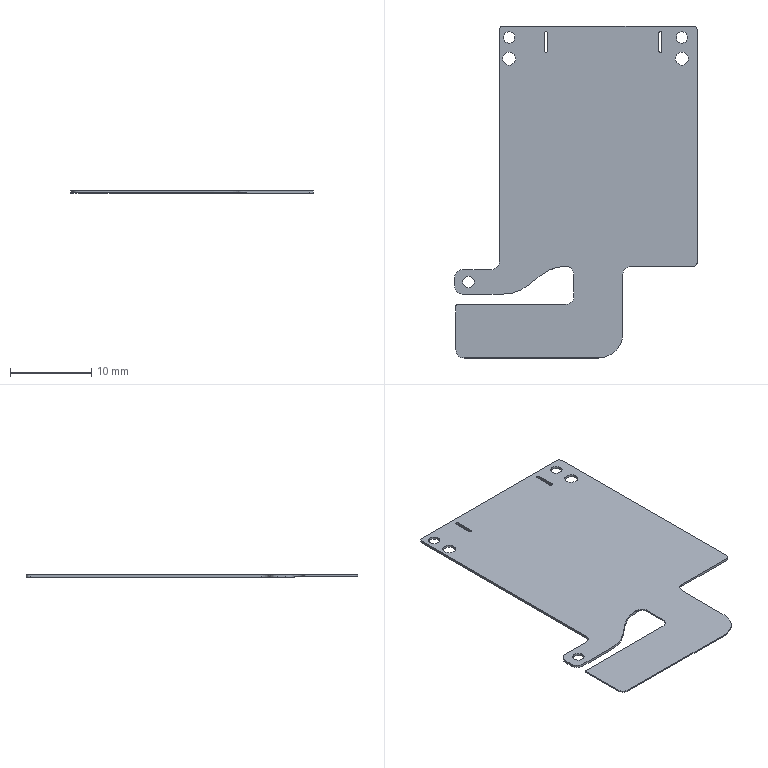Part | Creo | 1 solid | 48 faces | box 29.8 x 40.77 x 0.3 mm | volume 245.433 mm3 | cylinder 28 | plane 20 | commonest cylinder face diameters 2 x7 1.4 x6 0.4 x5 1.6 x4 1 x3 10 x2